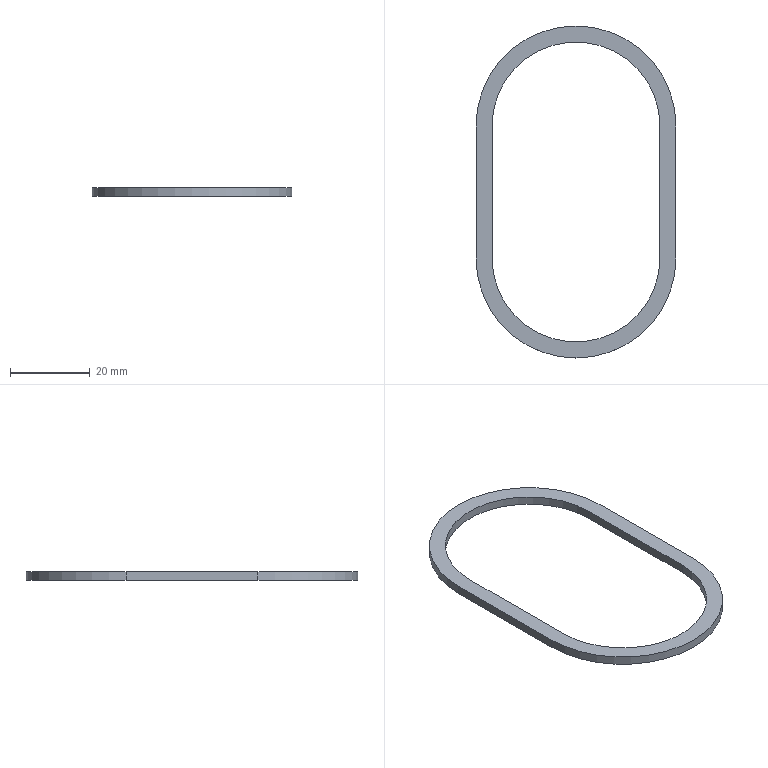Part | SolidWorks | features Extrusion 1 | 1 solid | 10 faces | box 50 x 83 x 2.2 mm | volume 1853 mm3 | plane 6 | cylinder 4 | commonest cylinder face diameters 42 x2 50 x2
STEP:
#1=CARTESIAN_POINT('',(-25.,0.,2.2));
#2=VERTEX_POINT('',#1);
#3=CARTESIAN_POINT('',(25.,0.,2.2));
#4=VERTEX_POINT('',#3);
#5=CARTESIAN_POINT('',(0.,0.,2.2));
#6=DIRECTION('',(0.,0.,1.));
#7=DIRECTION('',(1.,0.,0.));
#8=AXIS2_PLACEMENT_3D('',#5,#6,#7);
#9=CIRCLE('',#8,25.);
#10=EDGE_CURVE('',#2,#4,#9,.T.);
#11=ORIENTED_EDGE('',*,*,#10,.T.);
#12=CARTESIAN_POINT('',(25.,33.,2.2));
#13=VERTEX_POINT('',#12);
#14=CARTESIAN_POINT('',(25.,0.,2.2));
#15=DIRECTION('',(0.,1.,0.));
#16=VECTOR('',#15,1000.);
#17=LINE('',#14,#16);
#18=EDGE_CURVE('',#4,#13,#17,.T.);
#19=ORIENTED_EDGE('',*,*,#18,.T.);
#20=CARTESIAN_POINT('',(-25.,33.,2.2));
#21=VERTEX_POINT('',#20);
#22=CARTESIAN_POINT('',(0.,33.,2.2));
#23=DIRECTION('',(0.,0.,1.));
#24=DIRECTION('',(1.,0.,0.));
#25=AXIS2_PLACEMENT_3D('',#22,#23,#24);
#26=CIRCLE('',#25,25.);
#27=EDGE_CURVE('',#13,#21,#26,.T.);
#28=ORIENTED_EDGE('',*,*,#27,.T.);
#29=CARTESIAN_POINT('',(-25.,0.,2.2));
#30=DIRECTION('',(0.,-1.,0.));
#31=VECTOR('',#30,1000.);
#32=LINE('',#29,#31);
#33=EDGE_CURVE('',#21,#2,#32,.T.);
#34=ORIENTED_EDGE('',*,*,#33,.T.);
#35=EDGE_LOOP('',(#11,#19,#28,#34));
#36=FACE_OUTER_BOUND('',#35,.T.);
#37=CARTESIAN_POINT('',(21.,0.,2.2));
#38=VERTEX_POINT('',#37);
#39=CARTESIAN_POINT('',(21.,33.,2.2));
#40=VERTEX_POINT('',#39);
#41=CARTESIAN_POINT('',(21.,0.,2.2));
#42=DIRECTION('',(0.,1.,0.));
#43=VECTOR('',#42,1000.);
#44=LINE('',#41,#43);
#45=EDGE_CURVE('',#38,#40,#44,.T.);
#46=ORIENTED_EDGE('',*,*,#45,.F.);
#47=CARTESIAN_POINT('',(-21.,0.,2.2));
#48=VERTEX_POINT('',#47);
#49=CARTESIAN_POINT('',(0.,0.,2.2));
#50=DIRECTION('',(0.,0.,1.));
#51=DIRECTION('',(1.,0.,0.));
#52=AXIS2_PLACEMENT_3D('',#49,#50,#51);
#53=CIRCLE('',#52,21.);
#54=EDGE_CURVE('',#48,#38,#53,.T.);
#55=ORIENTED_EDGE('',*,*,#54,.F.);
#56=CARTESIAN_POINT('',(-21.,33.,2.2));
#57=VERTEX_POINT('',#56);
#58=CARTESIAN_POINT('',(-21.,0.,2.2));
#59=DIRECTION('',(0.,-1.,0.));
#60=VECTOR('',#59,1000.);
#61=LINE('',#58,#60);
#62=EDGE_CURVE('',#57,#48,#61,.T.);
#63=ORIENTED_EDGE('',*,*,#62,.F.);
#64=CARTESIAN_POINT('',(0.,33.,2.2));
#65=DIRECTION('',(0.,0.,1.));
#66=DIRECTION('',(1.,0.,0.));
#67=AXIS2_PLACEMENT_3D('',#64,#65,#66);
#68=CIRCLE('',#67,21.);
#69=EDGE_CURVE('',#40,#57,#68,.T.);
#70=ORIENTED_EDGE('',*,*,#69,.F.);
#71=EDGE_LOOP('',(#46,#55,#63,#70));
#72=FACE_BOUND('',#71,.T.);
#73=CARTESIAN_POINT('',(0.,0.,2.2));
#74=DIRECTION('',(0.,0.,1.));
#75=DIRECTION('',(1.,0.,0.));
#76=AXIS2_PLACEMENT_3D('',#73,#74,#75);
#77=PLANE('',#76);
#78=ADVANCED_FACE('',(#36,#72),#77,.T.);
#79=CARTESIAN_POINT('',(-25.,0.,0.));
#80=VERTEX_POINT('',#79);
#81=CARTESIAN_POINT('',(25.,0.,0.));
#82=VERTEX_POINT('',#81);
#83=CARTESIAN_POINT('',(0.,0.,0.));
#84=DIRECTION('',(0.,0.,1.));
#85=DIRECTION('',(1.,0.,0.));
#86=AXIS2_PLACEMENT_3D('',#83,#84,#85);
#87=CIRCLE('',#86,25.);
#88=EDGE_CURVE('',#80,#82,#87,.T.);
#89=ORIENTED_EDGE('',*,*,#88,.F.);
#90=CARTESIAN_POINT('',(-25.,33.,0.));
#91=VERTEX_POINT('',#90);
#92=CARTESIAN_POINT('',(-25.,0.,0.));
#93=DIRECTION('',(0.,-1.,0.));
#94=VECTOR('',#93,1000.);
#95=LINE('',#92,#94);
#96=EDGE_CURVE('',#91,#80,#95,.T.);
#97=ORIENTED_EDGE('',*,*,#96,.F.);
#98=CARTESIAN_POINT('',(25.,33.,0.));
#99=VERTEX_POINT('',#98);
#100=CARTESIAN_POINT('',(0.,33.,0.));
#101=DIRECTION('',(0.,0.,1.));
#102=DIRECTION('',(1.,0.,0.));
#103=AXIS2_PLACEMENT_3D('',#100,#101,#102);
#104=CIRCLE('',#103,25.);
#105=EDGE_CURVE('',#99,#91,#104,.T.);
#106=ORIENTED_EDGE('',*,*,#105,.F.);
#107=CARTESIAN_POINT('',(25.,0.,0.));
#108=DIRECTION('',(0.,1.,0.));
#109=VECTOR('',#108,1000.);
#110=LINE('',#107,#109);
#111=EDGE_CURVE('',#82,#99,#110,.T.);
#112=ORIENTED_EDGE('',*,*,#111,.F.);
#113=EDGE_LOOP('',(#89,#97,#106,#112));
#114=FACE_OUTER_BOUND('',#113,.T.);
#115=CARTESIAN_POINT('',(-21.,0.,0.));
#116=VERTEX_POINT('',#115);
#117=CARTESIAN_POINT('',(21.,0.,0.));
#118=VERTEX_POINT('',#117);
#119=CARTESIAN_POINT('',(0.,0.,0.));
#120=DIRECTION('',(0.,0.,1.));
#121=DIRECTION('',(1.,0.,0.));
#122=AXIS2_PLACEMENT_3D('',#119,#120,#121);
#123=CIRCLE('',#122,21.);
#124=EDGE_CURVE('',#116,#118,#123,.T.);
#125=ORIENTED_EDGE('',*,*,#124,.T.);
#126=CARTESIAN_POINT('',(21.,33.,0.));
#127=VERTEX_POINT('',#126);
#128=CARTESIAN_POINT('',(21.,0.,0.));
#129=DIRECTION('',(0.,1.,0.));
#130=VECTOR('',#129,1000.);
#131=LINE('',#128,#130);
#132=EDGE_CURVE('',#118,#127,#131,.T.);
#133=ORIENTED_EDGE('',*,*,#132,.T.);
#134=CARTESIAN_POINT('',(-21.,33.,0.));
#135=VERTEX_POINT('',#134);
#136=CARTESIAN_POINT('',(0.,33.,0.));
#137=DIRECTION('',(0.,0.,1.));
#138=DIRECTION('',(1.,0.,0.));
#139=AXIS2_PLACEMENT_3D('',#136,#137,#138);
#140=CIRCLE('',#139,21.);
#141=EDGE_CURVE('',#127,#135,#140,.T.);
#142=ORIENTED_EDGE('',*,*,#141,.T.);
#143=CARTESIAN_POINT('',(-21.,0.,0.));
#144=DIRECTION('',(0.,-1.,0.));
#145=VECTOR('',#144,1000.);
#146=LINE('',#143,#145);
#147=EDGE_CURVE('',#135,#116,#146,.T.);
#148=ORIENTED_EDGE('',*,*,#147,.T.);
#149=EDGE_LOOP('',(#125,#133,#142,#148));
#150=FACE_BOUND('',#149,.T.);
#151=CARTESIAN_POINT('',(0.,0.,0.));
#152=DIRECTION('',(0.,0.,1.));
#153=DIRECTION('',(1.,0.,0.));
#154=AXIS2_PLACEMENT_3D('',#151,#152,#153);
#155=PLANE('',#154);
#156=ADVANCED_FACE('',(#114,#150),#155,.F.);
#157=ORIENTED_EDGE('',*,*,#88,.T.);
#158=CARTESIAN_POINT('',(25.,0.,2.2));
#159=DIRECTION('',(0.,0.,-1.));
#160=VECTOR('',#159,1000.);
#161=LINE('',#158,#160);
#162=EDGE_CURVE('',#4,#82,#161,.T.);
#163=ORIENTED_EDGE('',*,*,#162,.F.);
#164=ORIENTED_EDGE('',*,*,#10,.F.);
#165=CARTESIAN_POINT('',(-25.,0.,2.2));
#166=DIRECTION('',(0.,0.,-1.));
#167=VECTOR('',#166,1000.);
#168=LINE('',#165,#167);
#169=EDGE_CURVE('',#2,#80,#168,.T.);
#170=ORIENTED_EDGE('',*,*,#169,.T.);
#171=EDGE_LOOP('',(#157,#163,#164,#170));
#172=FACE_OUTER_BOUND('',#171,.T.);
#173=CARTESIAN_POINT('',(0.,0.,2.2));
#174=DIRECTION('',(0.,0.,-1.));
#175=DIRECTION('',(-1.,0.,0.));
#176=AXIS2_PLACEMENT_3D('',#173,#174,#175);
#177=CYLINDRICAL_SURFACE('',#176,25.);
#178=ADVANCED_FACE('',(#172),#177,.T.);
#179=ORIENTED_EDGE('',*,*,#111,.T.);
#180=CARTESIAN_POINT('',(25.,33.,2.2));
#181=DIRECTION('',(0.,0.,-1.));
#182=VECTOR('',#181,1000.);
#183=LINE('',#180,#182);
#184=EDGE_CURVE('',#13,#99,#183,.T.);
#185=ORIENTED_EDGE('',*,*,#184,.F.);
#186=ORIENTED_EDGE('',*,*,#18,.F.);
#187=ORIENTED_EDGE('',*,*,#162,.T.);
#188=EDGE_LOOP('',(#179,#185,#186,#187));
#189=FACE_OUTER_BOUND('',#188,.T.);
#190=CARTESIAN_POINT('',(25.,0.,2.2));
#191=DIRECTION('',(-1.,0.,0.));
#192=DIRECTION('',(0.,0.,1.));
#193=AXIS2_PLACEMENT_3D('',#190,#191,#192);
#194=PLANE('',#193);
#195=ADVANCED_FACE('',(#189),#194,.F.);
#196=ORIENTED_EDGE('',*,*,#105,.T.);
#197=CARTESIAN_POINT('',(-25.,33.,2.2));
#198=DIRECTION('',(0.,0.,-1.));
#199=VECTOR('',#198,1000.);
#200=LINE('',#197,#199);
#201=EDGE_CURVE('',#21,#91,#200,.T.);
#202=ORIENTED_EDGE('',*,*,#201,.F.);
#203=ORIENTED_EDGE('',*,*,#27,.F.);
#204=ORIENTED_EDGE('',*,*,#184,.T.);
#205=EDGE_LOOP('',(#196,#202,#203,#204));
#206=FACE_OUTER_BOUND('',#205,.T.);
#207=CARTESIAN_POINT('',(0.,33.,2.2));
#208=DIRECTION('',(0.,0.,-1.));
#209=DIRECTION('',(-1.,0.,0.));
#210=AXIS2_PLACEMENT_3D('',#207,#208,#209);
#211=CYLINDRICAL_SURFACE('',#210,25.);
#212=ADVANCED_FACE('',(#206),#211,.T.);
#213=ORIENTED_EDGE('',*,*,#96,.T.);
#214=ORIENTED_EDGE('',*,*,#169,.F.);
#215=ORIENTED_EDGE('',*,*,#33,.F.);
#216=ORIENTED_EDGE('',*,*,#201,.T.);
#217=EDGE_LOOP('',(#213,#214,#215,#216));
#218=FACE_OUTER_BOUND('',#217,.T.);
#219=CARTESIAN_POINT('',(-25.,0.,2.2));
#220=DIRECTION('',(1.,0.,0.));
#221=DIRECTION('',(0.,0.,-1.));
#222=AXIS2_PLACEMENT_3D('',#219,#220,#221);
#223=PLANE('',#222);
#224=ADVANCED_FACE('',(#218),#223,.F.);
#225=ORIENTED_EDGE('',*,*,#124,.F.);
#226=CARTESIAN_POINT('',(-21.,0.,2.2));
#227=DIRECTION('',(0.,0.,-1.));
#228=VECTOR('',#227,1000.);
#229=LINE('',#226,#228);
#230=EDGE_CURVE('',#48,#116,#229,.T.);
#231=ORIENTED_EDGE('',*,*,#230,.F.);
#232=ORIENTED_EDGE('',*,*,#54,.T.);
#233=CARTESIAN_POINT('',(21.,0.,2.2));
#234=DIRECTION('',(0.,0.,-1.));
#235=VECTOR('',#234,1000.);
#236=LINE('',#233,#235);
#237=EDGE_CURVE('',#38,#118,#236,.T.);
#238=ORIENTED_EDGE('',*,*,#237,.T.);
#239=EDGE_LOOP('',(#225,#231,#232,#238));
#240=FACE_OUTER_BOUND('',#239,.T.);
#241=CARTESIAN_POINT('',(0.,0.,2.2));
#242=DIRECTION('',(0.,0.,-1.));
#243=DIRECTION('',(-1.,0.,0.));
#244=AXIS2_PLACEMENT_3D('',#241,#242,#243);
#245=CYLINDRICAL_SURFACE('',#244,21.);
#246=ADVANCED_FACE('',(#240),#245,.F.);
#247=ORIENTED_EDGE('',*,*,#132,.F.);
#248=ORIENTED_EDGE('',*,*,#237,.F.);
#249=ORIENTED_EDGE('',*,*,#45,.T.);
#250=CARTESIAN_POINT('',(21.,33.,2.2));
#251=DIRECTION('',(0.,0.,-1.));
#252=VECTOR('',#251,1000.);
#253=LINE('',#250,#252);
#254=EDGE_CURVE('',#40,#127,#253,.T.);
#255=ORIENTED_EDGE('',*,*,#254,.T.);
#256=EDGE_LOOP('',(#247,#248,#249,#255));
#257=FACE_OUTER_BOUND('',#256,.T.);
#258=CARTESIAN_POINT('',(21.,0.,2.2));
#259=DIRECTION('',(-1.,0.,0.));
#260=DIRECTION('',(0.,0.,1.));
#261=AXIS2_PLACEMENT_3D('',#258,#259,#260);
#262=PLANE('',#261);
#263=ADVANCED_FACE('',(#257),#262,.T.);
#264=ORIENTED_EDGE('',*,*,#141,.F.);
#265=ORIENTED_EDGE('',*,*,#254,.F.);
#266=ORIENTED_EDGE('',*,*,#69,.T.);
#267=CARTESIAN_POINT('',(-21.,33.,2.2));
#268=DIRECTION('',(0.,0.,-1.));
#269=VECTOR('',#268,1000.);
#270=LINE('',#267,#269);
#271=EDGE_CURVE('',#57,#135,#270,.T.);
#272=ORIENTED_EDGE('',*,*,#271,.T.);
#273=EDGE_LOOP('',(#264,#265,#266,#272));
#274=FACE_OUTER_BOUND('',#273,.T.);
#275=CARTESIAN_POINT('',(0.,33.,2.2));
#276=DIRECTION('',(0.,0.,-1.));
#277=DIRECTION('',(-1.,0.,0.));
#278=AXIS2_PLACEMENT_3D('',#275,#276,#277);
#279=CYLINDRICAL_SURFACE('',#278,21.);
#280=ADVANCED_FACE('',(#274),#279,.F.);
#281=ORIENTED_EDGE('',*,*,#147,.F.);
#282=ORIENTED_EDGE('',*,*,#271,.F.);
#283=ORIENTED_EDGE('',*,*,#62,.T.);
#284=ORIENTED_EDGE('',*,*,#230,.T.);
#285=EDGE_LOOP('',(#281,#282,#283,#284));
#286=FACE_OUTER_BOUND('',#285,.T.);
#287=CARTESIAN_POINT('',(-21.,0.,2.2));
#288=DIRECTION('',(1.,0.,0.));
#289=DIRECTION('',(0.,0.,-1.));
#290=AXIS2_PLACEMENT_3D('',#287,#288,#289);
#291=PLANE('',#290);
#292=ADVANCED_FACE('',(#286),#291,.T.);
#293=CLOSED_SHELL('',(#78,#156,#178,#195,#212,#224,#246,#263,#280,#292));
#294=MANIFOLD_SOLID_BREP('',#293);
#295=CARTESIAN_POINT('',(0.,0.,0.));
#296=DIRECTION('',(0.,0.,1.));
#297=DIRECTION('',(1.,0.,0.));
#298=AXIS2_PLACEMENT_3D('',#295,#296,#297);
#299=(LENGTH_UNIT()NAMED_UNIT(*)SI_UNIT(.MILLI.,.METRE.));
#300=UNCERTAINTY_MEASURE_WITH_UNIT(LENGTH_MEASURE(0.00001),#299,'','');
#301=(NAMED_UNIT(*)PLANE_ANGLE_UNIT()SI_UNIT($,.RADIAN.));
#302=(NAMED_UNIT(*)SI_UNIT($,.STERADIAN.)SOLID_ANGLE_UNIT());
#303=(GEOMETRIC_REPRESENTATION_CONTEXT(3)GLOBAL_UNCERTAINTY_ASSIGNED_CONTEXT((#300))GLOBAL_UNIT_ASSIGNED_CONTEXT((#299,#301,#302))REPRESENTATION_CONTEXT('',''));
#304=ADVANCED_BREP_SHAPE_REPRESENTATION('',(#294,#298),#303);